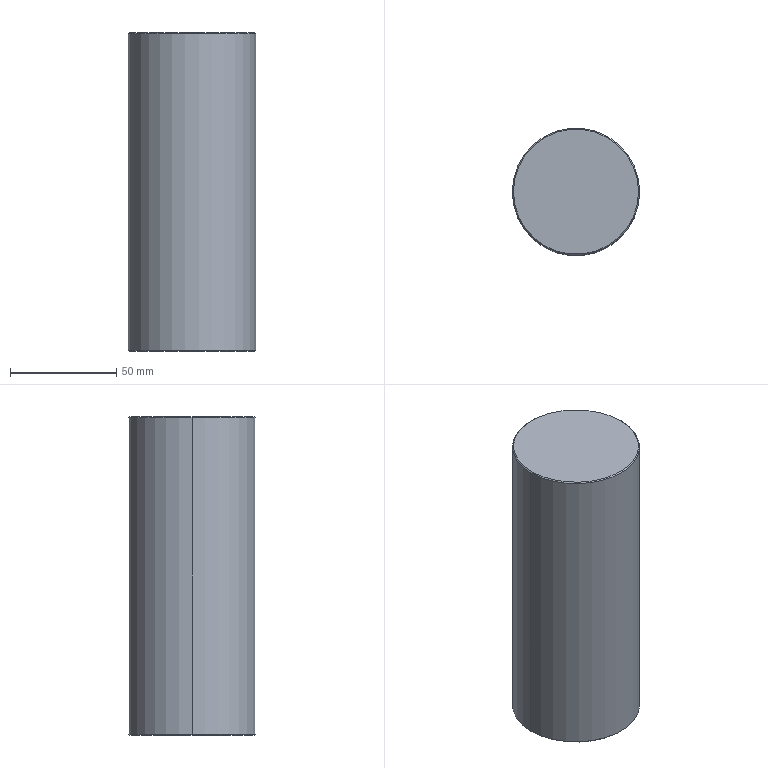Part | Creo | 1 solid | 12 faces | box 60 x 60 x 150 mm | volume 423275 mm3 | cone 6 | cylinder 4 | plane 2 | commonest cylinder face diameters 8 x2 60 x2
STEP:
#1=CARTESIAN_POINT('',(22.5,148.,-300.5));
#2=VERTEX_POINT('',#1);
#3=CARTESIAN_POINT('',(81.5,148.,-300.5));
#4=VERTEX_POINT('',#3);
#5=CARTESIAN_POINT('',(52.,148.,-300.5));
#6=DIRECTION('',(0.,0.,-1.));
#7=DIRECTION('',(-1.,0.,0.));
#8=AXIS2_PLACEMENT_3D('',#5,#6,#7);
#9=CIRCLE('',#8,29.5);
#10=EDGE_CURVE('',#2,#4,#9,.T.);
#11=ORIENTED_EDGE('',*,*,#10,.F.);
#12=CARTESIAN_POINT('',(52.,148.,-300.5));
#13=DIRECTION('',(0.,0.,-1.));
#14=DIRECTION('',(1.,0.,0.));
#15=AXIS2_PLACEMENT_3D('',#12,#13,#14);
#16=CIRCLE('',#15,29.5);
#17=EDGE_CURVE('',#4,#2,#16,.T.);
#18=ORIENTED_EDGE('',*,*,#17,.F.);
#19=EDGE_LOOP('',(#11,#18));
#20=FACE_OUTER_BOUND('',#19,.F.);
#21=CARTESIAN_POINT('',(56.,148.,-300.5));
#22=VERTEX_POINT('',#21);
#23=CARTESIAN_POINT('',(48.,148.,-300.5));
#24=VERTEX_POINT('',#23);
#25=CARTESIAN_POINT('',(52.,148.,-300.5));
#26=DIRECTION('',(0.,0.,1.));
#27=DIRECTION('',(1.,0.,0.));
#28=AXIS2_PLACEMENT_3D('',#25,#26,#27);
#29=CIRCLE('',#28,4.);
#30=EDGE_CURVE('',#22,#24,#29,.T.);
#31=ORIENTED_EDGE('',*,*,#30,.F.);
#32=CARTESIAN_POINT('',(52.,148.,-300.5));
#33=DIRECTION('',(0.,0.,1.));
#34=DIRECTION('',(-1.,0.,0.));
#35=AXIS2_PLACEMENT_3D('',#32,#33,#34);
#36=CIRCLE('',#35,4.);
#37=EDGE_CURVE('',#24,#22,#36,.T.);
#38=ORIENTED_EDGE('',*,*,#37,.F.);
#39=EDGE_LOOP('',(#31,#38));
#40=FACE_BOUND('',#39,.F.);
#41=CARTESIAN_POINT('',(52.,148.,-300.5));
#42=DIRECTION('',(0.,0.,-1.));
#43=DIRECTION('',(-1.,0.,0.));
#44=AXIS2_PLACEMENT_3D('',#41,#42,#43);
#45=PLANE('',#44);
#46=ADVANCED_FACE('',(#20,#40),#45,.T.);
#47=ORIENTED_EDGE('',*,*,#10,.T.);
#48=CARTESIAN_POINT('',(82.,148.,-300.));
#49=VERTEX_POINT('',#48);
#50=CARTESIAN_POINT('',(81.5,148.,-300.5));
#51=DIRECTION('',(0.7071,0.,0.7071));
#52=VECTOR('',#51,0.7071);
#53=LINE('',#50,#52);
#54=EDGE_CURVE('',#4,#49,#53,.T.);
#55=ORIENTED_EDGE('',*,*,#54,.T.);
#56=CARTESIAN_POINT('',(22.,148.,-300.));
#57=VERTEX_POINT('',#56);
#58=CARTESIAN_POINT('',(52.,148.,-300.));
#59=DIRECTION('',(0.,0.,-1.));
#60=DIRECTION('',(-1.,0.,0.));
#61=AXIS2_PLACEMENT_3D('',#58,#59,#60);
#62=CIRCLE('',#61,30.);
#63=EDGE_CURVE('',#57,#49,#62,.T.);
#64=ORIENTED_EDGE('',*,*,#63,.F.);
#65=CARTESIAN_POINT('',(22.5,148.,-300.5));
#66=DIRECTION('',(-0.7071,0.,0.7071));
#67=VECTOR('',#66,0.7071);
#68=LINE('',#65,#67);
#69=EDGE_CURVE('',#2,#57,#68,.T.);
#70=ORIENTED_EDGE('',*,*,#69,.F.);
#71=EDGE_LOOP('',(#47,#55,#64,#70));
#72=FACE_OUTER_BOUND('',#71,.F.);
#73=CARTESIAN_POINT('',(52.,148.,-300.25));
#74=DIRECTION('',(0.,0.,1.));
#75=DIRECTION('',(1.,0.,0.));
#76=AXIS2_PLACEMENT_3D('',#73,#74,#75);
#77=CONICAL_SURFACE('',#76,29.75,45.);
#78=ADVANCED_FACE('',(#72),#77,.T.);
#79=ORIENTED_EDGE('',*,*,#17,.T.);
#80=ORIENTED_EDGE('',*,*,#69,.T.);
#81=CARTESIAN_POINT('',(52.,148.,-300.));
#82=DIRECTION('',(0.,0.,-1.));
#83=DIRECTION('',(1.,0.,0.));
#84=AXIS2_PLACEMENT_3D('',#81,#82,#83);
#85=CIRCLE('',#84,30.);
#86=EDGE_CURVE('',#49,#57,#85,.T.);
#87=ORIENTED_EDGE('',*,*,#86,.F.);
#88=ORIENTED_EDGE('',*,*,#54,.F.);
#89=EDGE_LOOP('',(#79,#80,#87,#88));
#90=FACE_OUTER_BOUND('',#89,.F.);
#91=CARTESIAN_POINT('',(52.,148.,-300.25));
#92=DIRECTION('',(0.,0.,1.));
#93=DIRECTION('',(1.,0.,0.));
#94=AXIS2_PLACEMENT_3D('',#91,#92,#93);
#95=CONICAL_SURFACE('',#94,29.75,45.);
#96=ADVANCED_FACE('',(#90),#95,.T.);
#97=ORIENTED_EDGE('',*,*,#86,.T.);
#98=CARTESIAN_POINT('',(22.,148.,-151.));
#99=VERTEX_POINT('',#98);
#100=CARTESIAN_POINT('',(22.,148.,-151.));
#101=DIRECTION('',(0.,0.,-1.));
#102=VECTOR('',#101,149.);
#103=LINE('',#100,#102);
#104=EDGE_CURVE('',#99,#57,#103,.T.);
#105=ORIENTED_EDGE('',*,*,#104,.F.);
#106=CARTESIAN_POINT('',(82.,148.,-151.));
#107=VERTEX_POINT('',#106);
#108=CARTESIAN_POINT('',(52.,148.,-151.));
#109=DIRECTION('',(0.,0.,1.));
#110=DIRECTION('',(-1.,0.,0.));
#111=AXIS2_PLACEMENT_3D('',#108,#109,#110);
#112=CIRCLE('',#111,30.);
#113=EDGE_CURVE('',#99,#107,#112,.T.);
#114=ORIENTED_EDGE('',*,*,#113,.T.);
#115=CARTESIAN_POINT('',(82.,148.,-151.));
#116=DIRECTION('',(0.,0.,-1.));
#117=VECTOR('',#116,149.);
#118=LINE('',#115,#117);
#119=EDGE_CURVE('',#107,#49,#118,.T.);
#120=ORIENTED_EDGE('',*,*,#119,.T.);
#121=EDGE_LOOP('',(#97,#105,#114,#120));
#122=FACE_OUTER_BOUND('',#121,.F.);
#123=CARTESIAN_POINT('',(52.,148.,-150.5));
#124=DIRECTION('',(0.,0.,-1.));
#125=DIRECTION('',(-1.,0.,0.));
#126=AXIS2_PLACEMENT_3D('',#123,#124,#125);
#127=CYLINDRICAL_SURFACE('',#126,30.);
#128=ADVANCED_FACE('',(#122),#127,.T.);
#129=ORIENTED_EDGE('',*,*,#63,.T.);
#130=ORIENTED_EDGE('',*,*,#119,.F.);
#131=CARTESIAN_POINT('',(52.,148.,-151.));
#132=DIRECTION('',(0.,0.,1.));
#133=DIRECTION('',(1.,0.,0.));
#134=AXIS2_PLACEMENT_3D('',#131,#132,#133);
#135=CIRCLE('',#134,30.);
#136=EDGE_CURVE('',#107,#99,#135,.T.);
#137=ORIENTED_EDGE('',*,*,#136,.T.);
#138=ORIENTED_EDGE('',*,*,#104,.T.);
#139=EDGE_LOOP('',(#129,#130,#137,#138));
#140=FACE_OUTER_BOUND('',#139,.F.);
#141=CARTESIAN_POINT('',(52.,148.,-150.5));
#142=DIRECTION('',(0.,0.,-1.));
#143=DIRECTION('',(-1.,0.,0.));
#144=AXIS2_PLACEMENT_3D('',#141,#142,#143);
#145=CYLINDRICAL_SURFACE('',#144,30.);
#146=ADVANCED_FACE('',(#140),#145,.T.);
#147=CARTESIAN_POINT('',(81.5,148.,-150.5));
#148=VERTEX_POINT('',#147);
#149=CARTESIAN_POINT('',(22.5,148.,-150.5));
#150=VERTEX_POINT('',#149);
#151=CARTESIAN_POINT('',(52.,148.,-150.5));
#152=DIRECTION('',(0.,0.,1.));
#153=DIRECTION('',(1.,0.,0.));
#154=AXIS2_PLACEMENT_3D('',#151,#152,#153);
#155=CIRCLE('',#154,29.5);
#156=EDGE_CURVE('',#148,#150,#155,.T.);
#157=ORIENTED_EDGE('',*,*,#156,.T.);
#158=CARTESIAN_POINT('',(22.5,148.,-150.5));
#159=DIRECTION('',(-0.7071,0.,-0.7071));
#160=VECTOR('',#159,0.7071);
#161=LINE('',#158,#160);
#162=EDGE_CURVE('',#150,#99,#161,.T.);
#163=ORIENTED_EDGE('',*,*,#162,.T.);
#164=ORIENTED_EDGE('',*,*,#136,.F.);
#165=CARTESIAN_POINT('',(81.5,148.,-150.5));
#166=DIRECTION('',(0.7071,0.,-0.7071));
#167=VECTOR('',#166,0.7071);
#168=LINE('',#165,#167);
#169=EDGE_CURVE('',#148,#107,#168,.T.);
#170=ORIENTED_EDGE('',*,*,#169,.F.);
#171=EDGE_LOOP('',(#157,#163,#164,#170));
#172=FACE_OUTER_BOUND('',#171,.F.);
#173=CARTESIAN_POINT('',(52.,148.,-150.75));
#174=DIRECTION('',(0.,0.,-1.));
#175=DIRECTION('',(-1.,0.,0.));
#176=AXIS2_PLACEMENT_3D('',#173,#174,#175);
#177=CONICAL_SURFACE('',#176,29.75,45.);
#178=ADVANCED_FACE('',(#172),#177,.T.);
#179=ORIENTED_EDGE('',*,*,#156,.F.);
#180=CARTESIAN_POINT('',(52.,148.,-150.5));
#181=DIRECTION('',(0.,0.,1.));
#182=DIRECTION('',(-1.,0.,0.));
#183=AXIS2_PLACEMENT_3D('',#180,#181,#182);
#184=CIRCLE('',#183,29.5);
#185=EDGE_CURVE('',#150,#148,#184,.T.);
#186=ORIENTED_EDGE('',*,*,#185,.F.);
#187=EDGE_LOOP('',(#179,#186));
#188=FACE_OUTER_BOUND('',#187,.F.);
#189=CARTESIAN_POINT('',(52.,148.,-150.5));
#190=DIRECTION('',(0.,0.,1.));
#191=DIRECTION('',(1.,0.,0.));
#192=AXIS2_PLACEMENT_3D('',#189,#190,#191);
#193=PLANE('',#192);
#194=ADVANCED_FACE('',(#188),#193,.T.);
#195=ORIENTED_EDGE('',*,*,#185,.T.);
#196=ORIENTED_EDGE('',*,*,#169,.T.);
#197=ORIENTED_EDGE('',*,*,#113,.F.);
#198=ORIENTED_EDGE('',*,*,#162,.F.);
#199=EDGE_LOOP('',(#195,#196,#197,#198));
#200=FACE_OUTER_BOUND('',#199,.F.);
#201=CARTESIAN_POINT('',(52.,148.,-150.75));
#202=DIRECTION('',(0.,0.,-1.));
#203=DIRECTION('',(-1.,0.,0.));
#204=AXIS2_PLACEMENT_3D('',#201,#202,#203);
#205=CONICAL_SURFACE('',#204,29.75,45.);
#206=ADVANCED_FACE('',(#200),#205,.T.);
#207=CARTESIAN_POINT('',(48.,148.,-285.5));
#208=VERTEX_POINT('',#207);
#209=CARTESIAN_POINT('',(56.,148.,-285.5));
#210=VERTEX_POINT('',#209);
#211=CARTESIAN_POINT('',(52.,148.,-285.5));
#212=DIRECTION('',(0.,0.,-1.));
#213=DIRECTION('',(-1.,0.,0.));
#214=AXIS2_PLACEMENT_3D('',#211,#212,#213);
#215=CIRCLE('',#214,4.);
#216=EDGE_CURVE('',#208,#210,#215,.T.);
#217=ORIENTED_EDGE('',*,*,#216,.T.);
#218=CARTESIAN_POINT('',(56.,148.,-300.5));
#219=DIRECTION('',(0.,0.,1.));
#220=VECTOR('',#219,15.);
#221=LINE('',#218,#220);
#222=EDGE_CURVE('',#22,#210,#221,.T.);
#223=ORIENTED_EDGE('',*,*,#222,.F.);
#224=ORIENTED_EDGE('',*,*,#30,.T.);
#225=CARTESIAN_POINT('',(48.,148.,-300.5));
#226=DIRECTION('',(0.,0.,1.));
#227=VECTOR('',#226,15.);
#228=LINE('',#225,#227);
#229=EDGE_CURVE('',#24,#208,#228,.T.);
#230=ORIENTED_EDGE('',*,*,#229,.T.);
#231=EDGE_LOOP('',(#217,#223,#224,#230));
#232=FACE_OUTER_BOUND('',#231,.F.);
#233=CARTESIAN_POINT('',(52.,148.,-300.5));
#234=DIRECTION('',(0.,0.,1.));
#235=DIRECTION('',(1.,0.,0.));
#236=AXIS2_PLACEMENT_3D('',#233,#234,#235);
#237=CYLINDRICAL_SURFACE('',#236,4.);
#238=ADVANCED_FACE('',(#232),#237,.F.);
#239=ORIENTED_EDGE('',*,*,#216,.F.);
#240=CARTESIAN_POINT('',(52.,148.,-283.19));
#241=VERTEX_POINT('',#240);
#242=CARTESIAN_POINT('',(52.,148.,-283.19));
#243=DIRECTION('',(-0.866,0.,-0.5001));
#244=VECTOR('',#243,4.619);
#245=LINE('',#242,#244);
#246=EDGE_CURVE('',#241,#208,#245,.T.);
#247=ORIENTED_EDGE('',*,*,#246,.F.);
#248=CARTESIAN_POINT('',(52.,148.,-283.19));
#249=DIRECTION('',(0.866,0.,-0.5001));
#250=VECTOR('',#249,4.619);
#251=LINE('',#248,#250);
#252=EDGE_CURVE('',#241,#210,#251,.T.);
#253=ORIENTED_EDGE('',*,*,#252,.T.);
#254=EDGE_LOOP('',(#239,#247,#253));
#255=FACE_OUTER_BOUND('',#254,.F.);
#256=CARTESIAN_POINT('',(52.,148.,-284.397));
#257=DIRECTION('',(0.,0.,-1.));
#258=DIRECTION('',(-1.,0.,0.));
#259=AXIS2_PLACEMENT_3D('',#256,#257,#258);
#260=CONICAL_SURFACE('',#259,2.09,59.994);
#261=ADVANCED_FACE('',(#255),#260,.F.);
#262=CARTESIAN_POINT('',(52.,148.,-285.5));
#263=DIRECTION('',(0.,0.,-1.));
#264=DIRECTION('',(1.,0.,0.));
#265=AXIS2_PLACEMENT_3D('',#262,#263,#264);
#266=CIRCLE('',#265,4.);
#267=EDGE_CURVE('',#210,#208,#266,.T.);
#268=ORIENTED_EDGE('',*,*,#267,.F.);
#269=ORIENTED_EDGE('',*,*,#252,.F.);
#270=ORIENTED_EDGE('',*,*,#246,.T.);
#271=EDGE_LOOP('',(#268,#269,#270));
#272=FACE_OUTER_BOUND('',#271,.F.);
#273=CARTESIAN_POINT('',(52.,148.,-284.397));
#274=DIRECTION('',(0.,0.,-1.));
#275=DIRECTION('',(-1.,0.,0.));
#276=AXIS2_PLACEMENT_3D('',#273,#274,#275);
#277=CONICAL_SURFACE('',#276,2.09,59.994);
#278=ADVANCED_FACE('',(#272),#277,.F.);
#279=ORIENTED_EDGE('',*,*,#267,.T.);
#280=ORIENTED_EDGE('',*,*,#229,.F.);
#281=ORIENTED_EDGE('',*,*,#37,.T.);
#282=ORIENTED_EDGE('',*,*,#222,.T.);
#283=EDGE_LOOP('',(#279,#280,#281,#282));
#284=FACE_OUTER_BOUND('',#283,.F.);
#285=CARTESIAN_POINT('',(52.,148.,-300.5));
#286=DIRECTION('',(0.,0.,1.));
#287=DIRECTION('',(1.,0.,0.));
#288=AXIS2_PLACEMENT_3D('',#285,#286,#287);
#289=CYLINDRICAL_SURFACE('',#288,4.);
#290=ADVANCED_FACE('',(#284),#289,.F.);
#291=CLOSED_SHELL('',(#46,#78,#96,#128,#146,#178,#194,#206,#238,#261,#278,#290));
#292=MANIFOLD_SOLID_BREP('',#291);
#293=(LENGTH_UNIT()NAMED_UNIT(*)SI_UNIT(.MILLI.,.METRE.));
#294=UNCERTAINTY_MEASURE_WITH_UNIT(LENGTH_MEASURE(0.01723),#293,'','');
#295=(NAMED_UNIT(*)PLANE_ANGLE_UNIT()SI_UNIT($,.RADIAN.));
#296=PLANE_ANGLE_MEASURE_WITH_UNIT(PLANE_ANGLE_MEASURE(0.01745),#295);
#297=(CONVERSION_BASED_UNIT('DEGREE',#296)NAMED_UNIT(*)PLANE_ANGLE_UNIT());
#298=(NAMED_UNIT(*)SI_UNIT($,.STERADIAN.)SOLID_ANGLE_UNIT());
#299=(GEOMETRIC_REPRESENTATION_CONTEXT(3)GLOBAL_UNCERTAINTY_ASSIGNED_CONTEXT((#294))GLOBAL_UNIT_ASSIGNED_CONTEXT((#293,#297,#298))REPRESENTATION_CONTEXT('',''));
#300=ADVANCED_BREP_SHAPE_REPRESENTATION('',(#292),#299);